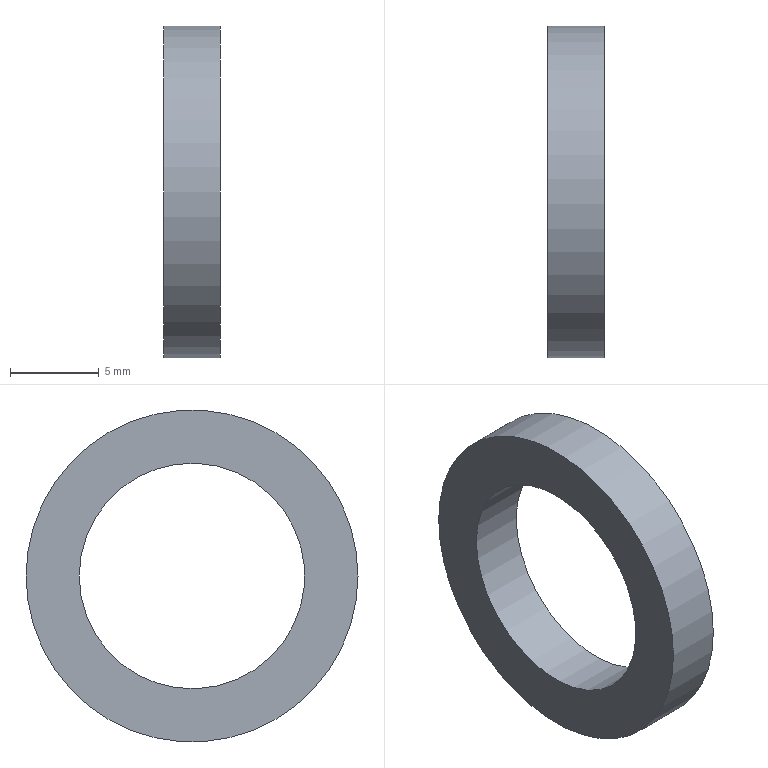Part | NX | features solid 2 | 1 solid | 4 faces | box 3.175 x 18.7 x 18.7 mm | volume 469.802 mm3 | cylinder 2 | plane 2 | commonest cylinder face diameters 12.7 x1 18.7 x1
STEP:
#1=CARTESIAN_POINT('',(3.175,9.35,0.));
#2=VERTEX_POINT('',#1);
#3=CARTESIAN_POINT('',(3.175,0.,0.));
#4=DIRECTION('',(1.,0.,0.));
#5=DIRECTION('',(0.,1.,0.));
#6=AXIS2_PLACEMENT_3D('',#3,#4,#5);
#7=CIRCLE('',#6,9.35);
#8=EDGE_CURVE('',#2,#2,#7,.T.);
#9=ORIENTED_EDGE('',*,*,#8,.F.);
#10=EDGE_LOOP('',(#9));
#11=FACE_BOUND('',#10,.T.);
#12=CARTESIAN_POINT('',(0.,9.35,0.));
#13=VERTEX_POINT('',#12);
#14=CARTESIAN_POINT('',(0.,0.,0.));
#15=DIRECTION('',(1.,0.,0.));
#16=DIRECTION('',(0.,1.,0.));
#17=AXIS2_PLACEMENT_3D('',#14,#15,#16);
#18=CIRCLE('',#17,9.35);
#19=EDGE_CURVE('',#13,#13,#18,.T.);
#20=ORIENTED_EDGE('',*,*,#19,.T.);
#21=EDGE_LOOP('',(#20));
#22=FACE_BOUND('',#21,.T.);
#23=CARTESIAN_POINT('',(3.175,0.,0.));
#24=DIRECTION('',(-1.,0.,0.));
#25=DIRECTION('',(0.,0.,1.));
#26=AXIS2_PLACEMENT_3D('',#23,#24,#25);
#27=CYLINDRICAL_SURFACE('',#26,9.35);
#28=ADVANCED_FACE('',(#11,#22),#27,.T.);
#29=CARTESIAN_POINT('',(3.175,6.35,0.));
#30=VERTEX_POINT('',#29);
#31=CARTESIAN_POINT('',(3.175,0.,0.));
#32=DIRECTION('',(1.,0.,0.));
#33=DIRECTION('',(0.,1.,0.));
#34=AXIS2_PLACEMENT_3D('',#31,#32,#33);
#35=CIRCLE('',#34,6.35);
#36=EDGE_CURVE('',#30,#30,#35,.F.);
#37=ORIENTED_EDGE('',*,*,#36,.F.);
#38=EDGE_LOOP('',(#37));
#39=FACE_BOUND('',#38,.T.);
#40=CARTESIAN_POINT('',(0.,6.35,0.));
#41=VERTEX_POINT('',#40);
#42=CARTESIAN_POINT('',(0.,0.,0.));
#43=DIRECTION('',(1.,0.,0.));
#44=DIRECTION('',(0.,1.,0.));
#45=AXIS2_PLACEMENT_3D('',#42,#43,#44);
#46=CIRCLE('',#45,6.35);
#47=EDGE_CURVE('',#41,#41,#46,.F.);
#48=ORIENTED_EDGE('',*,*,#47,.T.);
#49=EDGE_LOOP('',(#48));
#50=FACE_BOUND('',#49,.T.);
#51=CARTESIAN_POINT('',(3.175,0.,0.));
#52=DIRECTION('',(-1.,0.,0.));
#53=DIRECTION('',(0.,0.,1.));
#54=AXIS2_PLACEMENT_3D('',#51,#52,#53);
#55=CYLINDRICAL_SURFACE('',#54,6.35);
#56=ADVANCED_FACE('',(#39,#50),#55,.F.);
#57=ORIENTED_EDGE('',*,*,#8,.T.);
#58=EDGE_LOOP('',(#57));
#59=FACE_BOUND('',#58,.T.);
#60=ORIENTED_EDGE('',*,*,#36,.T.);
#61=EDGE_LOOP('',(#60));
#62=FACE_BOUND('',#61,.T.);
#63=CARTESIAN_POINT('',(3.175,0.,0.));
#64=DIRECTION('',(1.,0.,0.));
#65=DIRECTION('',(0.,0.,-1.));
#66=AXIS2_PLACEMENT_3D('',#63,#64,#65);
#67=PLANE('',#66);
#68=ADVANCED_FACE('',(#59,#62),#67,.T.);
#69=ORIENTED_EDGE('',*,*,#19,.F.);
#70=EDGE_LOOP('',(#69));
#71=FACE_BOUND('',#70,.T.);
#72=ORIENTED_EDGE('',*,*,#47,.F.);
#73=EDGE_LOOP('',(#72));
#74=FACE_BOUND('',#73,.T.);
#75=CARTESIAN_POINT('',(0.,0.,0.));
#76=DIRECTION('',(1.,0.,0.));
#77=DIRECTION('',(0.,0.,-1.));
#78=AXIS2_PLACEMENT_3D('',#75,#76,#77);
#79=PLANE('',#78);
#80=ADVANCED_FACE('',(#71,#74),#79,.F.);
#81=CLOSED_SHELL('',(#28,#56,#68,#80));
#82=MANIFOLD_SOLID_BREP('',#81);
#83=(LENGTH_UNIT()NAMED_UNIT(*)SI_UNIT(.MILLI.,.METRE.));
#84=UNCERTAINTY_MEASURE_WITH_UNIT(LENGTH_MEASURE(0.00001),#83,'','');
#85=(NAMED_UNIT(*)PLANE_ANGLE_UNIT()SI_UNIT($,.RADIAN.));
#86=(NAMED_UNIT(*)SI_UNIT($,.STERADIAN.)SOLID_ANGLE_UNIT());
#87=(GEOMETRIC_REPRESENTATION_CONTEXT(3)GLOBAL_UNCERTAINTY_ASSIGNED_CONTEXT((#84))GLOBAL_UNIT_ASSIGNED_CONTEXT((#83,#85,#86))REPRESENTATION_CONTEXT('',''));
#88=ADVANCED_BREP_SHAPE_REPRESENTATION('',(#82),#87);